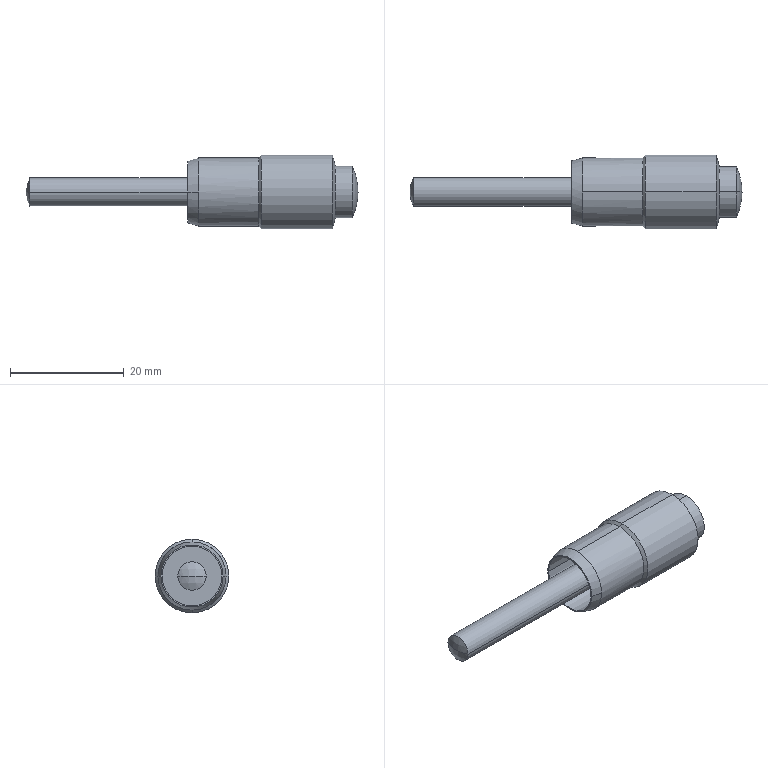Part | STEP file | Guide wheel mechanism revised.sldasm-Part-382 | 1 solid | 22 faces | box 58.5 x 13 x 13 mm | volume 2266 mm3 | cylinder 10 | cone 6 | sphere 2 | torus 2 | plane 2 | commonest cylinder face diameters 5 x2 9 x2 10.5 x2 11.995 x2 13 x2
STEP:
#1=CARTESIAN_POINT('',(-57.83,2.5,0.));
#2=VERTEX_POINT('',#1);
#3=CARTESIAN_POINT('',(-57.83,-2.5,0.));
#4=VERTEX_POINT('',#3);
#5=CARTESIAN_POINT('',(-57.83,0.,0.));
#6=DIRECTION('',(1.,0.,0.));
#7=DIRECTION('',(0.,1.,0.));
#8=AXIS2_PLACEMENT_3D('',#5,#6,#7);
#9=CIRCLE('',#8,2.5);
#10=EDGE_CURVE('',#2,#4,#9,.T.);
#11=ORIENTED_EDGE('',*,*,#10,.T.);
#12=CARTESIAN_POINT('',(-5.,-2.5,0.));
#13=VERTEX_POINT('',#12);
#14=CARTESIAN_POINT('',(-5.,-2.5,0.));
#15=DIRECTION('',(1.,0.,0.));
#16=VECTOR('',#15,1000.);
#17=LINE('',#14,#16);
#18=EDGE_CURVE('',#4,#13,#17,.T.);
#19=ORIENTED_EDGE('',*,*,#18,.T.);
#20=CARTESIAN_POINT('',(-5.,2.5,0.));
#21=VERTEX_POINT('',#20);
#22=CARTESIAN_POINT('',(-5.,0.,0.));
#23=DIRECTION('',(-1.,0.,0.));
#24=DIRECTION('',(0.,1.,0.));
#25=AXIS2_PLACEMENT_3D('',#22,#23,#24);
#26=CIRCLE('',#25,2.5);
#27=EDGE_CURVE('',#13,#21,#26,.T.);
#28=ORIENTED_EDGE('',*,*,#27,.T.);
#29=CARTESIAN_POINT('',(-5.,2.5,0.));
#30=DIRECTION('',(1.,0.,0.));
#31=VECTOR('',#30,1000.);
#32=LINE('',#29,#31);
#33=EDGE_CURVE('',#2,#21,#32,.T.);
#34=ORIENTED_EDGE('',*,*,#33,.F.);
#35=EDGE_LOOP('',(#11,#19,#28,#34));
#36=FACE_OUTER_BOUND('',#35,.T.);
#37=CARTESIAN_POINT('',(-5.,0.,0.));
#38=DIRECTION('',(1.,0.,0.));
#39=DIRECTION('',(0.,1.,0.));
#40=AXIS2_PLACEMENT_3D('',#37,#38,#39);
#41=CYLINDRICAL_SURFACE('',#40,2.5);
#42=ADVANCED_FACE('',(#36),#41,.T.);
#43=CARTESIAN_POINT('',(-57.83,0.,0.));
#44=DIRECTION('',(1.,0.,0.));
#45=DIRECTION('',(0.,1.,0.));
#46=AXIS2_PLACEMENT_3D('',#43,#44,#45);
#47=CIRCLE('',#46,2.5);
#48=EDGE_CURVE('',#4,#2,#47,.T.);
#49=ORIENTED_EDGE('',*,*,#48,.F.);
#50=CARTESIAN_POINT('',(-53.5,0.,0.));
#51=DIRECTION('',(0.,0.,-1.));
#52=DIRECTION('',(-1.,0.,0.));
#53=AXIS2_PLACEMENT_3D('',#50,#51,#52);
#54=CIRCLE('',#53,5.);
#55=EDGE_CURVE('',#4,#2,#54,.T.);
#56=ORIENTED_EDGE('',*,*,#55,.T.);
#57=EDGE_LOOP('',(#49,#56));
#58=FACE_OUTER_BOUND('',#57,.T.);
#59=CARTESIAN_POINT('',(-53.5,0.,0.));
#60=DIRECTION('',(0.,0.,1.));
#61=DIRECTION('',(-1.,0.,0.));
#62=AXIS2_PLACEMENT_3D('',#59,#60,#61);
#63=SPHERICAL_SURFACE('',#62,5.);
#64=ADVANCED_FACE('',(#58),#63,.T.);
#65=CARTESIAN_POINT('',(-5.,5.25,0.));
#66=VERTEX_POINT('',#65);
#67=CARTESIAN_POINT('',(-5.,-5.25,0.));
#68=VERTEX_POINT('',#67);
#69=CARTESIAN_POINT('',(-5.,0.,0.));
#70=DIRECTION('',(-1.,0.,0.));
#71=DIRECTION('',(0.,-1.,0.));
#72=AXIS2_PLACEMENT_3D('',#69,#70,#71);
#73=CIRCLE('',#72,5.25);
#74=EDGE_CURVE('',#66,#68,#73,.T.);
#75=ORIENTED_EDGE('',*,*,#74,.F.);
#76=CARTESIAN_POINT('',(-30.,5.25,0.));
#77=VERTEX_POINT('',#76);
#78=CARTESIAN_POINT('',(-5.,5.25,0.));
#79=DIRECTION('',(-1.,0.,0.));
#80=VECTOR('',#79,1000.);
#81=LINE('',#78,#80);
#82=EDGE_CURVE('',#66,#77,#81,.T.);
#83=ORIENTED_EDGE('',*,*,#82,.T.);
#84=CARTESIAN_POINT('',(-30.,-5.25,0.));
#85=VERTEX_POINT('',#84);
#86=CARTESIAN_POINT('',(-30.,0.,0.));
#87=DIRECTION('',(1.,0.,0.));
#88=DIRECTION('',(0.,-1.,0.));
#89=AXIS2_PLACEMENT_3D('',#86,#87,#88);
#90=CIRCLE('',#89,5.25);
#91=EDGE_CURVE('',#85,#77,#90,.T.);
#92=ORIENTED_EDGE('',*,*,#91,.F.);
#93=CARTESIAN_POINT('',(-5.,-5.25,0.));
#94=DIRECTION('',(-1.,0.,0.));
#95=VECTOR('',#94,1000.);
#96=LINE('',#93,#95);
#97=EDGE_CURVE('',#68,#85,#96,.T.);
#98=ORIENTED_EDGE('',*,*,#97,.F.);
#99=EDGE_LOOP('',(#75,#83,#92,#98));
#100=FACE_OUTER_BOUND('',#99,.T.);
#101=CARTESIAN_POINT('',(-5.,0.,0.));
#102=DIRECTION('',(-1.,0.,0.));
#103=DIRECTION('',(0.,-1.,0.));
#104=AXIS2_PLACEMENT_3D('',#101,#102,#103);
#105=CYLINDRICAL_SURFACE('',#104,5.25);
#106=ADVANCED_FACE('',(#100),#105,.F.);
#107=CARTESIAN_POINT('',(-30.,5.48,0.));
#108=VERTEX_POINT('',#107);
#109=CARTESIAN_POINT('',(-30.,-5.48,0.));
#110=VERTEX_POINT('',#109);
#111=CARTESIAN_POINT('',(-30.,0.,0.));
#112=DIRECTION('',(1.,0.,0.));
#113=DIRECTION('',(0.,1.,0.));
#114=AXIS2_PLACEMENT_3D('',#111,#112,#113);
#115=CIRCLE('',#114,5.48);
#116=EDGE_CURVE('',#108,#110,#115,.T.);
#117=ORIENTED_EDGE('',*,*,#116,.T.);
#118=CARTESIAN_POINT('',(-28.068,-5.998,0.));
#119=VERTEX_POINT('',#118);
#120=CARTESIAN_POINT('',(-28.068,-5.998,0.));
#121=DIRECTION('',(0.9659,-0.2588,0.));
#122=VECTOR('',#121,1000.);
#123=LINE('',#120,#122);
#124=EDGE_CURVE('',#110,#119,#123,.T.);
#125=ORIENTED_EDGE('',*,*,#124,.T.);
#126=CARTESIAN_POINT('',(-28.068,0.,5.998));
#127=VERTEX_POINT('',#126);
#128=CARTESIAN_POINT('',(-28.068,0.,0.));
#129=DIRECTION('',(-1.,0.,0.));
#130=DIRECTION('',(0.,0.,-1.));
#131=AXIS2_PLACEMENT_3D('',#128,#129,#130);
#132=CIRCLE('',#131,5.998);
#133=EDGE_CURVE('',#119,#127,#132,.T.);
#134=ORIENTED_EDGE('',*,*,#133,.T.);
#135=CARTESIAN_POINT('',(-28.068,5.998,0.));
#136=VERTEX_POINT('',#135);
#137=CARTESIAN_POINT('',(-28.068,0.,0.));
#138=DIRECTION('',(-1.,0.,0.));
#139=DIRECTION('',(0.,0.,-1.));
#140=AXIS2_PLACEMENT_3D('',#137,#138,#139);
#141=CIRCLE('',#140,5.998);
#142=EDGE_CURVE('',#127,#136,#141,.T.);
#143=ORIENTED_EDGE('',*,*,#142,.T.);
#144=CARTESIAN_POINT('',(-28.068,5.998,0.));
#145=DIRECTION('',(0.9659,0.2588,0.));
#146=VECTOR('',#145,1000.);
#147=LINE('',#144,#146);
#148=EDGE_CURVE('',#108,#136,#147,.T.);
#149=ORIENTED_EDGE('',*,*,#148,.F.);
#150=EDGE_LOOP('',(#117,#125,#134,#143,#149));
#151=FACE_OUTER_BOUND('',#150,.T.);
#152=CARTESIAN_POINT('',(-28.068,0.,0.));
#153=DIRECTION('',(1.,0.,0.));
#154=DIRECTION('',(0.,1.,0.));
#155=AXIS2_PLACEMENT_3D('',#152,#153,#154);
#156=CONICAL_SURFACE('',#155,5.998,0.2618);
#157=ADVANCED_FACE('',(#151),#156,.T.);
#158=CARTESIAN_POINT('',(-17.498,0.,5.998));
#159=VERTEX_POINT('',#158);
#160=CARTESIAN_POINT('',(-17.498,0.,-5.998));
#161=VERTEX_POINT('',#160);
#162=CARTESIAN_POINT('',(-17.498,0.,0.));
#163=DIRECTION('',(-1.,0.,0.));
#164=DIRECTION('',(0.,0.,1.));
#165=AXIS2_PLACEMENT_3D('',#162,#163,#164);
#166=CIRCLE('',#165,5.998);
#167=EDGE_CURVE('',#159,#161,#166,.T.);
#168=ORIENTED_EDGE('',*,*,#167,.T.);
#169=CARTESIAN_POINT('',(-28.068,0.,-5.998));
#170=VERTEX_POINT('',#169);
#171=CARTESIAN_POINT('',(-30.,0.,-5.998));
#172=DIRECTION('',(-1.,0.,0.));
#173=VECTOR('',#172,1000.);
#174=LINE('',#171,#173);
#175=EDGE_CURVE('',#161,#170,#174,.T.);
#176=ORIENTED_EDGE('',*,*,#175,.T.);
#177=CARTESIAN_POINT('',(-28.068,0.,0.));
#178=DIRECTION('',(-1.,0.,0.));
#179=DIRECTION('',(0.,0.,-1.));
#180=AXIS2_PLACEMENT_3D('',#177,#178,#179);
#181=CIRCLE('',#180,5.998);
#182=EDGE_CURVE('',#136,#170,#181,.T.);
#183=ORIENTED_EDGE('',*,*,#182,.F.);
#184=ORIENTED_EDGE('',*,*,#142,.F.);
#185=CARTESIAN_POINT('',(-30.,0.,5.998));
#186=DIRECTION('',(-1.,0.,0.));
#187=VECTOR('',#186,1000.);
#188=LINE('',#185,#187);
#189=EDGE_CURVE('',#159,#127,#188,.T.);
#190=ORIENTED_EDGE('',*,*,#189,.F.);
#191=EDGE_LOOP('',(#168,#176,#183,#184,#190));
#192=FACE_OUTER_BOUND('',#191,.T.);
#193=CARTESIAN_POINT('',(-30.,0.,0.));
#194=DIRECTION('',(-1.,0.,0.));
#195=DIRECTION('',(0.,0.,1.));
#196=AXIS2_PLACEMENT_3D('',#193,#194,#195);
#197=CYLINDRICAL_SURFACE('',#196,5.998);
#198=ADVANCED_FACE('',(#192),#197,.T.);
#199=ORIENTED_EDGE('',*,*,#167,.F.);
#200=CARTESIAN_POINT('',(-16.998,0.,6.5));
#201=VERTEX_POINT('',#200);
#202=CARTESIAN_POINT('',(-16.998,0.,6.5));
#203=DIRECTION('',(0.7054,0.,0.7088));
#204=VECTOR('',#203,1000.);
#205=LINE('',#202,#204);
#206=EDGE_CURVE('',#159,#201,#205,.T.);
#207=ORIENTED_EDGE('',*,*,#206,.T.);
#208=CARTESIAN_POINT('',(-16.998,0.,-6.5));
#209=VERTEX_POINT('',#208);
#210=CARTESIAN_POINT('',(-16.998,0.,0.));
#211=DIRECTION('',(-1.,0.,0.));
#212=DIRECTION('',(0.,0.,-1.));
#213=AXIS2_PLACEMENT_3D('',#210,#211,#212);
#214=CIRCLE('',#213,6.5);
#215=EDGE_CURVE('',#201,#209,#214,.T.);
#216=ORIENTED_EDGE('',*,*,#215,.T.);
#217=CARTESIAN_POINT('',(-16.998,0.,-6.5));
#218=DIRECTION('',(0.7054,0.,-0.7088));
#219=VECTOR('',#218,1000.);
#220=LINE('',#217,#219);
#221=EDGE_CURVE('',#161,#209,#220,.T.);
#222=ORIENTED_EDGE('',*,*,#221,.F.);
#223=EDGE_LOOP('',(#199,#207,#216,#222));
#224=FACE_OUTER_BOUND('',#223,.T.);
#225=CARTESIAN_POINT('',(-16.998,0.,0.));
#226=DIRECTION('',(1.,0.,0.));
#227=DIRECTION('',(0.,0.,-1.));
#228=AXIS2_PLACEMENT_3D('',#225,#226,#227);
#229=CONICAL_SURFACE('',#228,6.5,0.7878);
#230=ADVANCED_FACE('',(#224),#229,.T.);
#231=CARTESIAN_POINT('',(-4.498,0.,6.5));
#232=VERTEX_POINT('',#231);
#233=CARTESIAN_POINT('',(-4.498,0.,-6.5));
#234=VERTEX_POINT('',#233);
#235=CARTESIAN_POINT('',(-4.498,0.,0.));
#236=DIRECTION('',(-1.,0.,0.));
#237=DIRECTION('',(0.,0.,1.));
#238=AXIS2_PLACEMENT_3D('',#235,#236,#237);
#239=CIRCLE('',#238,6.5);
#240=EDGE_CURVE('',#232,#234,#239,.T.);
#241=ORIENTED_EDGE('',*,*,#240,.T.);
#242=CARTESIAN_POINT('',(-30.,0.,-6.5));
#243=DIRECTION('',(-1.,0.,0.));
#244=VECTOR('',#243,1000.);
#245=LINE('',#242,#244);
#246=EDGE_CURVE('',#234,#209,#245,.T.);
#247=ORIENTED_EDGE('',*,*,#246,.T.);
#248=ORIENTED_EDGE('',*,*,#215,.F.);
#249=CARTESIAN_POINT('',(-30.,0.,6.5));
#250=DIRECTION('',(-1.,0.,0.));
#251=VECTOR('',#250,1000.);
#252=LINE('',#249,#251);
#253=EDGE_CURVE('',#232,#201,#252,.T.);
#254=ORIENTED_EDGE('',*,*,#253,.F.);
#255=EDGE_LOOP('',(#241,#247,#248,#254));
#256=FACE_OUTER_BOUND('',#255,.T.);
#257=CARTESIAN_POINT('',(-30.,0.,0.));
#258=DIRECTION('',(-1.,0.,0.));
#259=DIRECTION('',(0.,0.,1.));
#260=AXIS2_PLACEMENT_3D('',#257,#258,#259);
#261=CYLINDRICAL_SURFACE('',#260,6.5);
#262=ADVANCED_FACE('',(#256),#261,.T.);
#263=CARTESIAN_POINT('',(-3.998,0.,4.5));
#264=VERTEX_POINT('',#263);
#265=CARTESIAN_POINT('',(-3.998,0.,-4.5));
#266=VERTEX_POINT('',#265);
#267=CARTESIAN_POINT('',(-3.998,0.,0.));
#268=DIRECTION('',(-1.,0.,0.));
#269=DIRECTION('',(0.,0.,1.));
#270=AXIS2_PLACEMENT_3D('',#267,#268,#269);
#271=CIRCLE('',#270,4.5);
#272=EDGE_CURVE('',#264,#266,#271,.T.);
#273=ORIENTED_EDGE('',*,*,#272,.T.);
#274=CARTESIAN_POINT('',(-4.498,0.,-6.5));
#275=DIRECTION('',(-0.2425,0.,-0.9701));
#276=VECTOR('',#275,1000.);
#277=LINE('',#274,#276);
#278=EDGE_CURVE('',#266,#234,#277,.T.);
#279=ORIENTED_EDGE('',*,*,#278,.T.);
#280=ORIENTED_EDGE('',*,*,#240,.F.);
#281=CARTESIAN_POINT('',(-4.498,0.,6.5));
#282=DIRECTION('',(-0.2425,0.,0.9701));
#283=VECTOR('',#282,1000.);
#284=LINE('',#281,#283);
#285=EDGE_CURVE('',#264,#232,#284,.T.);
#286=ORIENTED_EDGE('',*,*,#285,.F.);
#287=EDGE_LOOP('',(#273,#279,#280,#286));
#288=FACE_OUTER_BOUND('',#287,.T.);
#289=CARTESIAN_POINT('',(-4.498,0.,0.));
#290=DIRECTION('',(-1.,0.,0.));
#291=DIRECTION('',(0.,0.,1.));
#292=AXIS2_PLACEMENT_3D('',#289,#290,#291);
#293=CONICAL_SURFACE('',#292,6.5,1.326);
#294=ADVANCED_FACE('',(#288),#293,.T.);
#295=CARTESIAN_POINT('',(-0.9981,0.,4.5));
#296=VERTEX_POINT('',#295);
#297=CARTESIAN_POINT('',(-0.9981,0.,-4.5));
#298=VERTEX_POINT('',#297);
#299=CARTESIAN_POINT('',(-0.9981,0.,0.));
#300=DIRECTION('',(-1.,0.,0.));
#301=DIRECTION('',(0.,0.,1.));
#302=AXIS2_PLACEMENT_3D('',#299,#300,#301);
#303=CIRCLE('',#302,4.5);
#304=EDGE_CURVE('',#296,#298,#303,.T.);
#305=ORIENTED_EDGE('',*,*,#304,.T.);
#306=CARTESIAN_POINT('',(-30.,0.,-4.5));
#307=DIRECTION('',(-1.,0.,0.));
#308=VECTOR('',#307,1000.);
#309=LINE('',#306,#308);
#310=EDGE_CURVE('',#298,#266,#309,.T.);
#311=ORIENTED_EDGE('',*,*,#310,.T.);
#312=ORIENTED_EDGE('',*,*,#272,.F.);
#313=CARTESIAN_POINT('',(-30.,0.,4.5));
#314=DIRECTION('',(-1.,0.,0.));
#315=VECTOR('',#314,1000.);
#316=LINE('',#313,#315);
#317=EDGE_CURVE('',#296,#264,#316,.T.);
#318=ORIENTED_EDGE('',*,*,#317,.F.);
#319=EDGE_LOOP('',(#305,#311,#312,#318));
#320=FACE_OUTER_BOUND('',#319,.T.);
#321=CARTESIAN_POINT('',(-30.,0.,0.));
#322=DIRECTION('',(-1.,0.,0.));
#323=DIRECTION('',(0.,0.,1.));
#324=AXIS2_PLACEMENT_3D('',#321,#322,#323);
#325=CYLINDRICAL_SURFACE('',#324,4.5);
#326=ADVANCED_FACE('',(#320),#325,.T.);
#327=CARTESIAN_POINT('',(0.,0.,0.));
#328=VERTEX_POINT('',#327);
#329=CARTESIAN_POINT('',(-10.5,0.,0.0317));
#330=DIRECTION('',(0.,-1.,0.));
#331=DIRECTION('',(0.,0.,-1.));
#332=AXIS2_PLACEMENT_3D('',#329,#330,#331);
#333=CIRCLE('',#332,10.5);
#334=EDGE_CURVE('',#328,#296,#333,.T.);
#335=ORIENTED_EDGE('',*,*,#334,.F.);
#336=CARTESIAN_POINT('',(-10.5,0.,-0.0317));
#337=DIRECTION('',(0.,1.,0.));
#338=DIRECTION('',(0.,0.,1.));
#339=AXIS2_PLACEMENT_3D('',#336,#337,#338);
#340=CIRCLE('',#339,10.5);
#341=EDGE_CURVE('',#328,#298,#340,.T.);
#342=ORIENTED_EDGE('',*,*,#341,.T.);
#343=ORIENTED_EDGE('',*,*,#304,.F.);
#344=EDGE_LOOP('',(#335,#342,#343));
#345=FACE_OUTER_BOUND('',#344,.T.);
#346=CARTESIAN_POINT('',(-10.5,0.,0.));
#347=DIRECTION('',(-1.,0.,0.));
#348=DIRECTION('',(0.,0.,1.));
#349=AXIS2_PLACEMENT_3D('',#346,#347,#348);
#350=TOROIDAL_SURFACE('',#349,0.0317,10.5);
#351=ADVANCED_FACE('',(#345),#350,.T.);
#352=ORIENTED_EDGE('',*,*,#18,.F.);
#353=ORIENTED_EDGE('',*,*,#48,.T.);
#354=ORIENTED_EDGE('',*,*,#33,.T.);
#355=CARTESIAN_POINT('',(-5.,0.,0.));
#356=DIRECTION('',(-1.,0.,0.));
#357=DIRECTION('',(0.,1.,0.));
#358=AXIS2_PLACEMENT_3D('',#355,#356,#357);
#359=CIRCLE('',#358,2.5);
#360=EDGE_CURVE('',#21,#13,#359,.T.);
#361=ORIENTED_EDGE('',*,*,#360,.T.);
#362=EDGE_LOOP('',(#352,#353,#354,#361));
#363=FACE_OUTER_BOUND('',#362,.T.);
#364=CARTESIAN_POINT('',(-5.,0.,0.));
#365=DIRECTION('',(1.,0.,0.));
#366=DIRECTION('',(0.,1.,0.));
#367=AXIS2_PLACEMENT_3D('',#364,#365,#366);
#368=CYLINDRICAL_SURFACE('',#367,2.5);
#369=ADVANCED_FACE('',(#363),#368,.T.);
#370=ORIENTED_EDGE('',*,*,#360,.F.);
#371=ORIENTED_EDGE('',*,*,#27,.F.);
#372=EDGE_LOOP('',(#370,#371));
#373=FACE_BOUND('',#372,.T.);
#374=CARTESIAN_POINT('',(-5.,0.,0.));
#375=DIRECTION('',(-1.,0.,0.));
#376=DIRECTION('',(0.,-1.,0.));
#377=AXIS2_PLACEMENT_3D('',#374,#375,#376);
#378=CIRCLE('',#377,5.25);
#379=EDGE_CURVE('',#68,#66,#378,.T.);
#380=ORIENTED_EDGE('',*,*,#379,.T.);
#381=ORIENTED_EDGE('',*,*,#74,.T.);
#382=EDGE_LOOP('',(#380,#381));
#383=FACE_OUTER_BOUND('',#382,.T.);
#384=CARTESIAN_POINT('',(-5.,0.,0.));
#385=DIRECTION('',(-1.,0.,0.));
#386=DIRECTION('',(0.,-1.,0.));
#387=AXIS2_PLACEMENT_3D('',#384,#385,#386);
#388=PLANE('',#387);
#389=ADVANCED_FACE('',(#373,#383),#388,.T.);
#390=ORIENTED_EDGE('',*,*,#55,.F.);
#391=ORIENTED_EDGE('',*,*,#10,.F.);
#392=EDGE_LOOP('',(#390,#391));
#393=FACE_OUTER_BOUND('',#392,.T.);
#394=CARTESIAN_POINT('',(-53.5,0.,0.));
#395=DIRECTION('',(0.,0.,1.));
#396=DIRECTION('',(-1.,0.,0.));
#397=AXIS2_PLACEMENT_3D('',#394,#395,#396);
#398=SPHERICAL_SURFACE('',#397,5.);
#399=ADVANCED_FACE('',(#393),#398,.T.);
#400=ORIENTED_EDGE('',*,*,#82,.F.);
#401=ORIENTED_EDGE('',*,*,#379,.F.);
#402=ORIENTED_EDGE('',*,*,#97,.T.);
#403=CARTESIAN_POINT('',(-30.,0.,0.));
#404=DIRECTION('',(1.,0.,0.));
#405=DIRECTION('',(0.,-1.,0.));
#406=AXIS2_PLACEMENT_3D('',#403,#404,#405);
#407=CIRCLE('',#406,5.25);
#408=EDGE_CURVE('',#77,#85,#407,.T.);
#409=ORIENTED_EDGE('',*,*,#408,.F.);
#410=EDGE_LOOP('',(#400,#401,#402,#409));
#411=FACE_OUTER_BOUND('',#410,.T.);
#412=CARTESIAN_POINT('',(-5.,0.,0.));
#413=DIRECTION('',(-1.,0.,0.));
#414=DIRECTION('',(0.,-1.,0.));
#415=AXIS2_PLACEMENT_3D('',#412,#413,#414);
#416=CYLINDRICAL_SURFACE('',#415,5.25);
#417=ADVANCED_FACE('',(#411),#416,.F.);
#418=ORIENTED_EDGE('',*,*,#91,.T.);
#419=ORIENTED_EDGE('',*,*,#408,.T.);
#420=EDGE_LOOP('',(#418,#419));
#421=FACE_BOUND('',#420,.T.);
#422=ORIENTED_EDGE('',*,*,#116,.F.);
#423=CARTESIAN_POINT('',(-30.,0.,0.));
#424=DIRECTION('',(1.,0.,0.));
#425=DIRECTION('',(0.,1.,0.));
#426=AXIS2_PLACEMENT_3D('',#423,#424,#425);
#427=CIRCLE('',#426,5.48);
#428=EDGE_CURVE('',#110,#108,#427,.T.);
#429=ORIENTED_EDGE('',*,*,#428,.F.);
#430=EDGE_LOOP('',(#422,#429));
#431=FACE_OUTER_BOUND('',#430,.T.);
#432=CARTESIAN_POINT('',(-30.,0.,0.));
#433=DIRECTION('',(1.,0.,0.));
#434=DIRECTION('',(0.,0.,-1.));
#435=AXIS2_PLACEMENT_3D('',#432,#433,#434);
#436=PLANE('',#435);
#437=ADVANCED_FACE('',(#421,#431),#436,.F.);
#438=ORIENTED_EDGE('',*,*,#124,.F.);
#439=ORIENTED_EDGE('',*,*,#428,.T.);
#440=ORIENTED_EDGE('',*,*,#148,.T.);
#441=ORIENTED_EDGE('',*,*,#182,.T.);
#442=CARTESIAN_POINT('',(-28.068,0.,0.));
#443=DIRECTION('',(-1.,0.,0.));
#444=DIRECTION('',(0.,0.,-1.));
#445=AXIS2_PLACEMENT_3D('',#442,#443,#444);
#446=CIRCLE('',#445,5.998);
#447=EDGE_CURVE('',#170,#119,#446,.T.);
#448=ORIENTED_EDGE('',*,*,#447,.T.);
#449=EDGE_LOOP('',(#438,#439,#440,#441,#448));
#450=FACE_OUTER_BOUND('',#449,.T.);
#451=CARTESIAN_POINT('',(-28.068,0.,0.));
#452=DIRECTION('',(1.,0.,0.));
#453=DIRECTION('',(0.,1.,0.));
#454=AXIS2_PLACEMENT_3D('',#451,#452,#453);
#455=CONICAL_SURFACE('',#454,5.998,0.2618);
#456=ADVANCED_FACE('',(#450),#455,.T.);
#457=ORIENTED_EDGE('',*,*,#175,.F.);
#458=CARTESIAN_POINT('',(-17.498,0.,0.));
#459=DIRECTION('',(-1.,0.,0.));
#460=DIRECTION('',(0.,0.,1.));
#461=AXIS2_PLACEMENT_3D('',#458,#459,#460);
#462=CIRCLE('',#461,5.998);
#463=EDGE_CURVE('',#161,#159,#462,.T.);
#464=ORIENTED_EDGE('',*,*,#463,.T.);
#465=ORIENTED_EDGE('',*,*,#189,.T.);
#466=ORIENTED_EDGE('',*,*,#133,.F.);
#467=ORIENTED_EDGE('',*,*,#447,.F.);
#468=EDGE_LOOP('',(#457,#464,#465,#466,#467));
#469=FACE_OUTER_BOUND('',#468,.T.);
#470=CARTESIAN_POINT('',(-30.,0.,0.));
#471=DIRECTION('',(-1.,0.,0.));
#472=DIRECTION('',(0.,0.,1.));
#473=AXIS2_PLACEMENT_3D('',#470,#471,#472);
#474=CYLINDRICAL_SURFACE('',#473,5.998);
#475=ADVANCED_FACE('',(#469),#474,.T.);
#476=ORIENTED_EDGE('',*,*,#206,.F.);
#477=ORIENTED_EDGE('',*,*,#463,.F.);
#478=ORIENTED_EDGE('',*,*,#221,.T.);
#479=CARTESIAN_POINT('',(-16.998,0.,0.));
#480=DIRECTION('',(-1.,0.,0.));
#481=DIRECTION('',(0.,0.,-1.));
#482=AXIS2_PLACEMENT_3D('',#479,#480,#481);
#483=CIRCLE('',#482,6.5);
#484=EDGE_CURVE('',#209,#201,#483,.T.);
#485=ORIENTED_EDGE('',*,*,#484,.T.);
#486=EDGE_LOOP('',(#476,#477,#478,#485));
#487=FACE_OUTER_BOUND('',#486,.T.);
#488=CARTESIAN_POINT('',(-16.998,0.,0.));
#489=DIRECTION('',(1.,0.,0.));
#490=DIRECTION('',(0.,0.,-1.));
#491=AXIS2_PLACEMENT_3D('',#488,#489,#490);
#492=CONICAL_SURFACE('',#491,6.5,0.7878);
#493=ADVANCED_FACE('',(#487),#492,.T.);
#494=ORIENTED_EDGE('',*,*,#246,.F.);
#495=CARTESIAN_POINT('',(-4.498,0.,0.));
#496=DIRECTION('',(-1.,0.,0.));
#497=DIRECTION('',(0.,0.,1.));
#498=AXIS2_PLACEMENT_3D('',#495,#496,#497);
#499=CIRCLE('',#498,6.5);
#500=EDGE_CURVE('',#234,#232,#499,.T.);
#501=ORIENTED_EDGE('',*,*,#500,.T.);
#502=ORIENTED_EDGE('',*,*,#253,.T.);
#503=ORIENTED_EDGE('',*,*,#484,.F.);
#504=EDGE_LOOP('',(#494,#501,#502,#503));
#505=FACE_OUTER_BOUND('',#504,.T.);
#506=CARTESIAN_POINT('',(-30.,0.,0.));
#507=DIRECTION('',(-1.,0.,0.));
#508=DIRECTION('',(0.,0.,1.));
#509=AXIS2_PLACEMENT_3D('',#506,#507,#508);
#510=CYLINDRICAL_SURFACE('',#509,6.5);
#511=ADVANCED_FACE('',(#505),#510,.T.);
#512=ORIENTED_EDGE('',*,*,#278,.F.);
#513=CARTESIAN_POINT('',(-3.998,0.,0.));
#514=DIRECTION('',(-1.,0.,0.));
#515=DIRECTION('',(0.,0.,1.));
#516=AXIS2_PLACEMENT_3D('',#513,#514,#515);
#517=CIRCLE('',#516,4.5);
#518=EDGE_CURVE('',#266,#264,#517,.T.);
#519=ORIENTED_EDGE('',*,*,#518,.T.);
#520=ORIENTED_EDGE('',*,*,#285,.T.);
#521=ORIENTED_EDGE('',*,*,#500,.F.);
#522=EDGE_LOOP('',(#512,#519,#520,#521));
#523=FACE_OUTER_BOUND('',#522,.T.);
#524=CARTESIAN_POINT('',(-4.498,0.,0.));
#525=DIRECTION('',(-1.,0.,0.));
#526=DIRECTION('',(0.,0.,1.));
#527=AXIS2_PLACEMENT_3D('',#524,#525,#526);
#528=CONICAL_SURFACE('',#527,6.5,1.326);
#529=ADVANCED_FACE('',(#523),#528,.T.);
#530=ORIENTED_EDGE('',*,*,#310,.F.);
#531=CARTESIAN_POINT('',(-0.9981,0.,0.));
#532=DIRECTION('',(-1.,0.,0.));
#533=DIRECTION('',(0.,0.,1.));
#534=AXIS2_PLACEMENT_3D('',#531,#532,#533);
#535=CIRCLE('',#534,4.5);
#536=EDGE_CURVE('',#298,#296,#535,.T.);
#537=ORIENTED_EDGE('',*,*,#536,.T.);
#538=ORIENTED_EDGE('',*,*,#317,.T.);
#539=ORIENTED_EDGE('',*,*,#518,.F.);
#540=EDGE_LOOP('',(#530,#537,#538,#539));
#541=FACE_OUTER_BOUND('',#540,.T.);
#542=CARTESIAN_POINT('',(-30.,0.,0.));
#543=DIRECTION('',(-1.,0.,0.));
#544=DIRECTION('',(0.,0.,1.));
#545=AXIS2_PLACEMENT_3D('',#542,#543,#544);
#546=CYLINDRICAL_SURFACE('',#545,4.5);
#547=ADVANCED_FACE('',(#541),#546,.T.);
#548=ORIENTED_EDGE('',*,*,#341,.F.);
#549=ORIENTED_EDGE('',*,*,#334,.T.);
#550=ORIENTED_EDGE('',*,*,#536,.F.);
#551=EDGE_LOOP('',(#548,#549,#550));
#552=FACE_OUTER_BOUND('',#551,.T.);
#553=CARTESIAN_POINT('',(-10.5,0.,0.));
#554=DIRECTION('',(-1.,0.,0.));
#555=DIRECTION('',(0.,0.,1.));
#556=AXIS2_PLACEMENT_3D('',#553,#554,#555);
#557=TOROIDAL_SURFACE('',#556,0.0317,10.5);
#558=ADVANCED_FACE('',(#552),#557,.T.);
#559=CLOSED_SHELL('',(#42,#64,#106,#157,#198,#230,#262,#294,#326,#351,#369,#389,#399,#417,#437,#456,#475,#493,#511,#529,#547,#558));
#560=MANIFOLD_SOLID_BREP('',#559);
#561=CARTESIAN_POINT('',(0.,0.,0.));
#562=DIRECTION('',(0.,0.,1.));
#563=DIRECTION('',(1.,0.,0.));
#564=AXIS2_PLACEMENT_3D('',#561,#562,#563);
#565=(LENGTH_UNIT()NAMED_UNIT(*)SI_UNIT(.MILLI.,.METRE.));
#566=UNCERTAINTY_MEASURE_WITH_UNIT(LENGTH_MEASURE(0.00001),#565,'','');
#567=(NAMED_UNIT(*)PLANE_ANGLE_UNIT()SI_UNIT($,.RADIAN.));
#568=(NAMED_UNIT(*)SI_UNIT($,.STERADIAN.)SOLID_ANGLE_UNIT());
#569=(GEOMETRIC_REPRESENTATION_CONTEXT(3)GLOBAL_UNCERTAINTY_ASSIGNED_CONTEXT((#566))GLOBAL_UNIT_ASSIGNED_CONTEXT((#565,#567,#568))REPRESENTATION_CONTEXT('',''));
#570=ADVANCED_BREP_SHAPE_REPRESENTATION('',(#560,#564),#569);